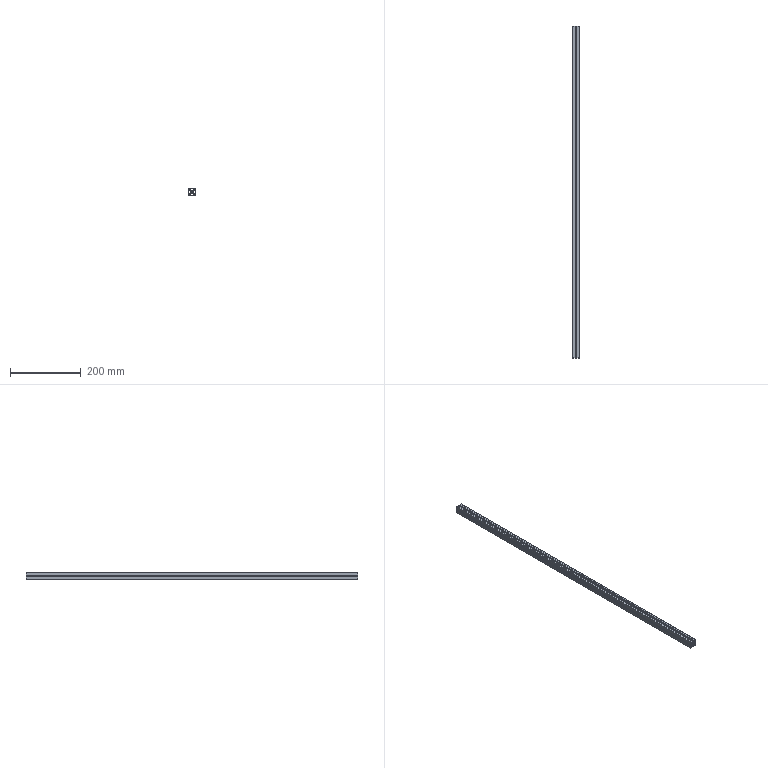Part | STEP file | 20 aluminium profile longitudinal 3 | 1 solid | 64 faces | box 20 x 940 x 20 mm | volume 167113 mm3 | plane 54 | cylinder 10 | commonest cylinder face diameters 3.3 x10